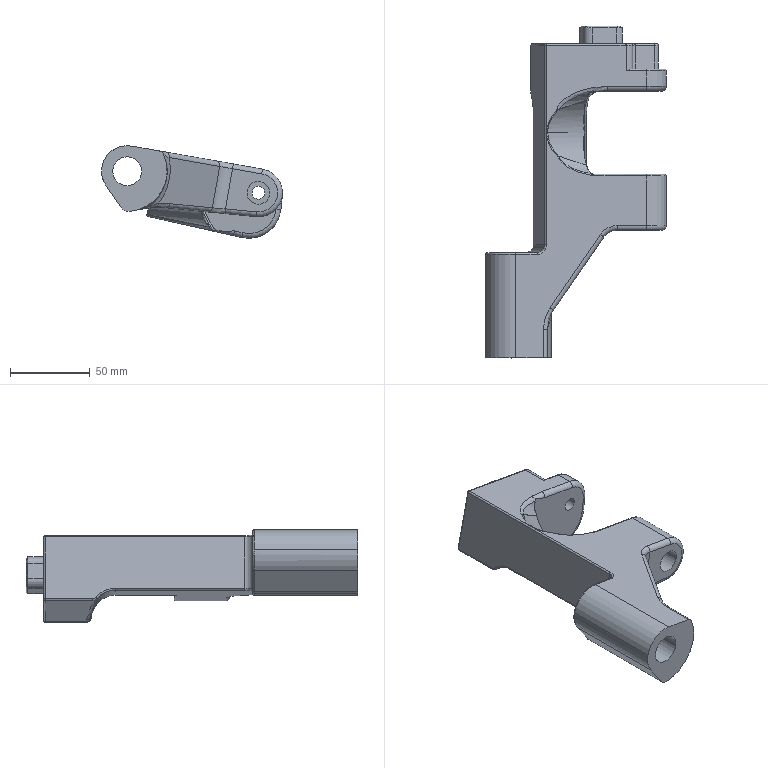Part | SolidWorks | features BaseBody 1 | 1 solid | 155 faces | box 113.061 x 207.5 x 57.89 mm | volume 321329 mm3 | cylinder 62 | plane 28 | spline 25 | torus 22 | cone 13 | sphere 5 | commonest cylinder face diameters 2 x16 6 x8 10 x8 8.5 x6 30 x5 7.95 x4